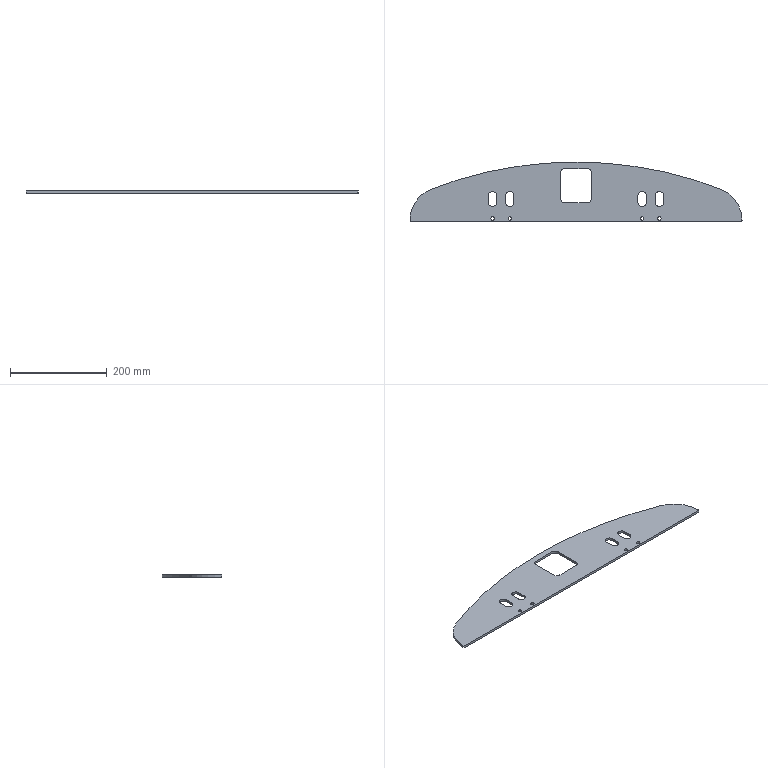Part | SolidWorks | features ICE 3, Fillet 1, FlatPattern 1, SMBaseFlange 1, SheetMetal 1 | 1 solid | 39 faces | box 688.178 x 124 x 5 mm | volume 305727 mm3 | cylinder 24 | plane 15 | commonest cylinder face diameters 7 x8 17 x8 20 x4 138.091 x3 1660 x1
STEP:
#1=CARTESIAN_POINT('',(230.5,7.,-5.));
#2=VERTEX_POINT('',#1);
#3=CARTESIAN_POINT('',(223.5,7.,-5.));
#4=VERTEX_POINT('',#3);
#5=CARTESIAN_POINT('',(227.,7.,-5.));
#6=DIRECTION('',(0.,0.,-1.));
#7=DIRECTION('',(-1.,0.,0.));
#8=AXIS2_PLACEMENT_3D('',#5,#6,#7);
#9=CIRCLE('',#8,3.5);
#10=EDGE_CURVE('',#2,#4,#9,.T.);
#11=ORIENTED_EDGE('',*,*,#10,.T.);
#12=CARTESIAN_POINT('',(223.5,7.,0.));
#13=VERTEX_POINT('',#12);
#14=CARTESIAN_POINT('',(223.5,7.,-10.));
#15=DIRECTION('',(0.,0.,1.));
#16=VECTOR('',#15,1000.);
#17=LINE('',#14,#16);
#18=EDGE_CURVE('',#4,#13,#17,.T.);
#19=ORIENTED_EDGE('',*,*,#18,.T.);
#20=CARTESIAN_POINT('',(230.5,7.,0.));
#21=VERTEX_POINT('',#20);
#22=CARTESIAN_POINT('',(227.,7.,0.));
#23=DIRECTION('',(0.,0.,1.));
#24=DIRECTION('',(1.,0.,0.));
#25=AXIS2_PLACEMENT_3D('',#22,#23,#24);
#26=CIRCLE('',#25,3.5);
#27=EDGE_CURVE('',#13,#21,#26,.T.);
#28=ORIENTED_EDGE('',*,*,#27,.T.);
#29=CARTESIAN_POINT('',(230.5,7.,-10.));
#30=DIRECTION('',(0.,0.,1.));
#31=VECTOR('',#30,1000.);
#32=LINE('',#29,#31);
#33=EDGE_CURVE('',#2,#21,#32,.T.);
#34=ORIENTED_EDGE('',*,*,#33,.F.);
#35=EDGE_LOOP('',(#11,#19,#28,#34));
#36=FACE_OUTER_BOUND('',#35,.T.);
#37=CARTESIAN_POINT('',(227.,7.,-10.));
#38=DIRECTION('',(0.,0.,1.));
#39=DIRECTION('',(1.,0.,0.));
#40=AXIS2_PLACEMENT_3D('',#37,#38,#39);
#41=CYLINDRICAL_SURFACE('',#40,3.5);
#42=ADVANCED_FACE('',(#36),#41,.F.);
#43=CARTESIAN_POINT('',(266.5,7.,-5.));
#44=VERTEX_POINT('',#43);
#45=CARTESIAN_POINT('',(259.5,7.,-5.));
#46=VERTEX_POINT('',#45);
#47=CARTESIAN_POINT('',(263.,7.,-5.));
#48=DIRECTION('',(0.,0.,-1.));
#49=DIRECTION('',(-1.,0.,0.));
#50=AXIS2_PLACEMENT_3D('',#47,#48,#49);
#51=CIRCLE('',#50,3.5);
#52=EDGE_CURVE('',#44,#46,#51,.T.);
#53=ORIENTED_EDGE('',*,*,#52,.T.);
#54=CARTESIAN_POINT('',(259.5,7.,0.));
#55=VERTEX_POINT('',#54);
#56=CARTESIAN_POINT('',(259.5,7.,-10.));
#57=DIRECTION('',(0.,0.,1.));
#58=VECTOR('',#57,1000.);
#59=LINE('',#56,#58);
#60=EDGE_CURVE('',#46,#55,#59,.T.);
#61=ORIENTED_EDGE('',*,*,#60,.T.);
#62=CARTESIAN_POINT('',(266.5,7.,0.));
#63=VERTEX_POINT('',#62);
#64=CARTESIAN_POINT('',(263.,7.,0.));
#65=DIRECTION('',(0.,0.,1.));
#66=DIRECTION('',(1.,0.,0.));
#67=AXIS2_PLACEMENT_3D('',#64,#65,#66);
#68=CIRCLE('',#67,3.5);
#69=EDGE_CURVE('',#55,#63,#68,.T.);
#70=ORIENTED_EDGE('',*,*,#69,.T.);
#71=CARTESIAN_POINT('',(266.5,7.,-10.));
#72=DIRECTION('',(0.,0.,1.));
#73=VECTOR('',#72,1000.);
#74=LINE('',#71,#73);
#75=EDGE_CURVE('',#44,#63,#74,.T.);
#76=ORIENTED_EDGE('',*,*,#75,.F.);
#77=EDGE_LOOP('',(#53,#61,#70,#76));
#78=FACE_OUTER_BOUND('',#77,.T.);
#79=CARTESIAN_POINT('',(263.,7.,-10.));
#80=DIRECTION('',(0.,0.,1.));
#81=DIRECTION('',(1.,0.,0.));
#82=AXIS2_PLACEMENT_3D('',#79,#80,#81);
#83=CYLINDRICAL_SURFACE('',#82,3.5);
#84=ADVANCED_FACE('',(#78),#83,.F.);
#85=CARTESIAN_POINT('',(540.5,7.,-5.));
#86=VERTEX_POINT('',#85);
#87=CARTESIAN_POINT('',(533.5,7.,-5.));
#88=VERTEX_POINT('',#87);
#89=CARTESIAN_POINT('',(537.,7.,-5.));
#90=DIRECTION('',(0.,0.,-1.));
#91=DIRECTION('',(-1.,0.,0.));
#92=AXIS2_PLACEMENT_3D('',#89,#90,#91);
#93=CIRCLE('',#92,3.5);
#94=EDGE_CURVE('',#86,#88,#93,.T.);
#95=ORIENTED_EDGE('',*,*,#94,.T.);
#96=CARTESIAN_POINT('',(533.5,7.,0.));
#97=VERTEX_POINT('',#96);
#98=CARTESIAN_POINT('',(533.5,7.,-10.));
#99=DIRECTION('',(0.,0.,1.));
#100=VECTOR('',#99,1000.);
#101=LINE('',#98,#100);
#102=EDGE_CURVE('',#88,#97,#101,.T.);
#103=ORIENTED_EDGE('',*,*,#102,.T.);
#104=CARTESIAN_POINT('',(540.5,7.,0.));
#105=VERTEX_POINT('',#104);
#106=CARTESIAN_POINT('',(537.,7.,0.));
#107=DIRECTION('',(0.,0.,1.));
#108=DIRECTION('',(-1.,0.,0.));
#109=AXIS2_PLACEMENT_3D('',#106,#107,#108);
#110=CIRCLE('',#109,3.5);
#111=EDGE_CURVE('',#97,#105,#110,.T.);
#112=ORIENTED_EDGE('',*,*,#111,.T.);
#113=CARTESIAN_POINT('',(540.5,7.,-10.));
#114=DIRECTION('',(0.,0.,1.));
#115=VECTOR('',#114,1000.);
#116=LINE('',#113,#115);
#117=EDGE_CURVE('',#86,#105,#116,.T.);
#118=ORIENTED_EDGE('',*,*,#117,.F.);
#119=EDGE_LOOP('',(#95,#103,#112,#118));
#120=FACE_OUTER_BOUND('',#119,.T.);
#121=CARTESIAN_POINT('',(537.,7.,-10.));
#122=DIRECTION('',(0.,0.,1.));
#123=DIRECTION('',(1.,0.,0.));
#124=AXIS2_PLACEMENT_3D('',#121,#122,#123);
#125=CYLINDRICAL_SURFACE('',#124,3.5);
#126=ADVANCED_FACE('',(#120),#125,.F.);
#127=CARTESIAN_POINT('',(576.5,7.,-5.));
#128=VERTEX_POINT('',#127);
#129=CARTESIAN_POINT('',(569.5,7.,-5.));
#130=VERTEX_POINT('',#129);
#131=CARTESIAN_POINT('',(573.,7.,-5.));
#132=DIRECTION('',(0.,0.,-1.));
#133=DIRECTION('',(-1.,0.,0.));
#134=AXIS2_PLACEMENT_3D('',#131,#132,#133);
#135=CIRCLE('',#134,3.5);
#136=EDGE_CURVE('',#128,#130,#135,.T.);
#137=ORIENTED_EDGE('',*,*,#136,.T.);
#138=CARTESIAN_POINT('',(569.5,7.,0.));
#139=VERTEX_POINT('',#138);
#140=CARTESIAN_POINT('',(569.5,7.,-10.));
#141=DIRECTION('',(0.,0.,1.));
#142=VECTOR('',#141,1000.);
#143=LINE('',#140,#142);
#144=EDGE_CURVE('',#130,#139,#143,.T.);
#145=ORIENTED_EDGE('',*,*,#144,.T.);
#146=CARTESIAN_POINT('',(576.5,7.,0.));
#147=VERTEX_POINT('',#146);
#148=CARTESIAN_POINT('',(573.,7.,0.));
#149=DIRECTION('',(0.,0.,1.));
#150=DIRECTION('',(-1.,0.,0.));
#151=AXIS2_PLACEMENT_3D('',#148,#149,#150);
#152=CIRCLE('',#151,3.5);
#153=EDGE_CURVE('',#139,#147,#152,.T.);
#154=ORIENTED_EDGE('',*,*,#153,.T.);
#155=CARTESIAN_POINT('',(576.5,7.,-10.));
#156=DIRECTION('',(0.,0.,1.));
#157=VECTOR('',#156,1000.);
#158=LINE('',#155,#157);
#159=EDGE_CURVE('',#128,#147,#158,.T.);
#160=ORIENTED_EDGE('',*,*,#159,.F.);
#161=EDGE_LOOP('',(#137,#145,#154,#160));
#162=FACE_OUTER_BOUND('',#161,.T.);
#163=CARTESIAN_POINT('',(573.,7.,-10.));
#164=DIRECTION('',(0.,0.,1.));
#165=DIRECTION('',(1.,0.,0.));
#166=AXIS2_PLACEMENT_3D('',#163,#164,#165);
#167=CYLINDRICAL_SURFACE('',#166,3.5);
#168=ADVANCED_FACE('',(#162),#167,.F.);
#169=CARTESIAN_POINT('',(744.,0.,-5.));
#170=VERTEX_POINT('',#169);
#171=CARTESIAN_POINT('',(744.089,3.509,-5.));
#172=VERTEX_POINT('',#171);
#173=CARTESIAN_POINT('',(675.044,3.509,-5.));
#174=DIRECTION('',(0.,0.,1.));
#175=DIRECTION('',(1.,0.,0.));
#176=AXIS2_PLACEMENT_3D('',#173,#174,#175);
#177=CIRCLE('',#176,69.045);
#178=EDGE_CURVE('',#170,#172,#177,.T.);
#179=ORIENTED_EDGE('',*,*,#178,.T.);
#180=CARTESIAN_POINT('',(744.089,3.509,0.));
#181=VERTEX_POINT('',#180);
#182=CARTESIAN_POINT('',(744.089,3.509,-5.));
#183=DIRECTION('',(0.,0.,1.));
#184=VECTOR('',#183,1000.);
#185=LINE('',#182,#184);
#186=EDGE_CURVE('',#172,#181,#185,.T.);
#187=ORIENTED_EDGE('',*,*,#186,.T.);
#188=CARTESIAN_POINT('',(744.,0.,0.));
#189=VERTEX_POINT('',#188);
#190=CARTESIAN_POINT('',(675.044,3.509,0.));
#191=DIRECTION('',(0.,0.,1.));
#192=DIRECTION('',(1.,0.,0.));
#193=AXIS2_PLACEMENT_3D('',#190,#191,#192);
#194=CIRCLE('',#193,69.045);
#195=EDGE_CURVE('',#189,#181,#194,.T.);
#196=ORIENTED_EDGE('',*,*,#195,.F.);
#197=CARTESIAN_POINT('',(744.,0.,-5.));
#198=DIRECTION('',(0.,0.,1.));
#199=VECTOR('',#198,1000.);
#200=LINE('',#197,#199);
#201=EDGE_CURVE('',#170,#189,#200,.T.);
#202=ORIENTED_EDGE('',*,*,#201,.F.);
#203=EDGE_LOOP('',(#179,#187,#196,#202));
#204=FACE_OUTER_BOUND('',#203,.T.);
#205=CARTESIAN_POINT('',(675.044,3.509,-5.));
#206=DIRECTION('',(0.,0.,1.));
#207=DIRECTION('',(1.,0.,0.));
#208=AXIS2_PLACEMENT_3D('',#205,#206,#207);
#209=CYLINDRICAL_SURFACE('',#208,69.045);
#210=ADVANCED_FACE('',(#204),#209,.T.);
#211=CARTESIAN_POINT('',(100.,67.886,0.));
#212=VERTEX_POINT('',#211);
#213=CARTESIAN_POINT('',(56.,0.,0.));
#214=VERTEX_POINT('',#213);
#215=CARTESIAN_POINT('',(124.956,3.509,0.));
#216=DIRECTION('',(0.,0.,1.));
#217=DIRECTION('',(-1.,0.,0.));
#218=AXIS2_PLACEMENT_3D('',#215,#216,#217);
#219=CIRCLE('',#218,69.045);
#220=EDGE_CURVE('',#212,#214,#219,.T.);
#221=ORIENTED_EDGE('',*,*,#220,.F.);
#222=CARTESIAN_POINT('',(100.,67.886,-5.));
#223=VERTEX_POINT('',#222);
#224=CARTESIAN_POINT('',(100.,67.886,-5.));
#225=DIRECTION('',(0.,0.,1.));
#226=VECTOR('',#225,1000.);
#227=LINE('',#224,#226);
#228=EDGE_CURVE('',#223,#212,#227,.T.);
#229=ORIENTED_EDGE('',*,*,#228,.F.);
#230=CARTESIAN_POINT('',(56.,0.,-5.));
#231=VERTEX_POINT('',#230);
#232=CARTESIAN_POINT('',(124.956,3.509,-5.));
#233=DIRECTION('',(0.,0.,1.));
#234=DIRECTION('',(-1.,0.,0.));
#235=AXIS2_PLACEMENT_3D('',#232,#233,#234);
#236=CIRCLE('',#235,69.045);
#237=EDGE_CURVE('',#223,#231,#236,.T.);
#238=ORIENTED_EDGE('',*,*,#237,.T.);
#239=CARTESIAN_POINT('',(56.,0.,-5.));
#240=DIRECTION('',(0.,0.,1.));
#241=VECTOR('',#240,1000.);
#242=LINE('',#239,#241);
#243=EDGE_CURVE('',#231,#214,#242,.T.);
#244=ORIENTED_EDGE('',*,*,#243,.T.);
#245=EDGE_LOOP('',(#221,#229,#238,#244));
#246=FACE_OUTER_BOUND('',#245,.T.);
#247=CARTESIAN_POINT('',(124.956,3.509,-5.));
#248=DIRECTION('',(0.,0.,1.));
#249=DIRECTION('',(1.,0.,0.));
#250=AXIS2_PLACEMENT_3D('',#247,#248,#249);
#251=CYLINDRICAL_SURFACE('',#250,69.045);
#252=ADVANCED_FACE('',(#246),#251,.T.);
#253=CARTESIAN_POINT('',(700.,67.886,0.));
#254=VERTEX_POINT('',#253);
#255=CARTESIAN_POINT('',(400.,-706.,0.));
#256=DIRECTION('',(0.,0.,1.));
#257=DIRECTION('',(-1.,0.,0.));
#258=AXIS2_PLACEMENT_3D('',#255,#256,#257);
#259=CIRCLE('',#258,830.);
#260=EDGE_CURVE('',#254,#212,#259,.T.);
#261=ORIENTED_EDGE('',*,*,#260,.F.);
#262=CARTESIAN_POINT('',(700.,67.886,-5.));
#263=VERTEX_POINT('',#262);
#264=CARTESIAN_POINT('',(700.,67.886,-5.));
#265=DIRECTION('',(0.,0.,1.));
#266=VECTOR('',#265,1000.);
#267=LINE('',#264,#266);
#268=EDGE_CURVE('',#263,#254,#267,.T.);
#269=ORIENTED_EDGE('',*,*,#268,.F.);
#270=CARTESIAN_POINT('',(400.,-706.,-5.));
#271=DIRECTION('',(0.,0.,1.));
#272=DIRECTION('',(-1.,0.,0.));
#273=AXIS2_PLACEMENT_3D('',#270,#271,#272);
#274=CIRCLE('',#273,830.);
#275=EDGE_CURVE('',#263,#223,#274,.T.);
#276=ORIENTED_EDGE('',*,*,#275,.T.);
#277=ORIENTED_EDGE('',*,*,#228,.T.);
#278=EDGE_LOOP('',(#261,#269,#276,#277));
#279=FACE_OUTER_BOUND('',#278,.T.);
#280=CARTESIAN_POINT('',(400.,-706.,-5.));
#281=DIRECTION('',(0.,0.,1.));
#282=DIRECTION('',(1.,0.,0.));
#283=AXIS2_PLACEMENT_3D('',#280,#281,#282);
#284=CYLINDRICAL_SURFACE('',#283,830.);
#285=ADVANCED_FACE('',(#279),#284,.T.);
#286=ORIENTED_EDGE('',*,*,#186,.F.);
#287=CARTESIAN_POINT('',(675.044,3.509,-5.));
#288=DIRECTION('',(0.,0.,1.));
#289=DIRECTION('',(1.,0.,0.));
#290=AXIS2_PLACEMENT_3D('',#287,#288,#289);
#291=CIRCLE('',#290,69.045);
#292=EDGE_CURVE('',#172,#263,#291,.T.);
#293=ORIENTED_EDGE('',*,*,#292,.T.);
#294=ORIENTED_EDGE('',*,*,#268,.T.);
#295=CARTESIAN_POINT('',(675.044,3.509,0.));
#296=DIRECTION('',(0.,0.,1.));
#297=DIRECTION('',(1.,0.,0.));
#298=AXIS2_PLACEMENT_3D('',#295,#296,#297);
#299=CIRCLE('',#298,69.045);
#300=EDGE_CURVE('',#181,#254,#299,.T.);
#301=ORIENTED_EDGE('',*,*,#300,.F.);
#302=EDGE_LOOP('',(#286,#293,#294,#301));
#303=FACE_OUTER_BOUND('',#302,.T.);
#304=CARTESIAN_POINT('',(675.044,3.509,-5.));
#305=DIRECTION('',(0.,0.,1.));
#306=DIRECTION('',(1.,0.,0.));
#307=AXIS2_PLACEMENT_3D('',#304,#305,#306);
#308=CYLINDRICAL_SURFACE('',#307,69.045);
#309=ADVANCED_FACE('',(#303),#308,.T.);
#310=CARTESIAN_POINT('',(56.,0.,0.));
#311=DIRECTION('',(1.,0.,0.));
#312=VECTOR('',#311,1000.);
#313=LINE('',#310,#312);
#314=EDGE_CURVE('',#214,#189,#313,.T.);
#315=ORIENTED_EDGE('',*,*,#314,.F.);
#316=ORIENTED_EDGE('',*,*,#243,.F.);
#317=CARTESIAN_POINT('',(56.,0.,-5.));
#318=DIRECTION('',(1.,0.,0.));
#319=VECTOR('',#318,1000.);
#320=LINE('',#317,#319);
#321=EDGE_CURVE('',#231,#170,#320,.T.);
#322=ORIENTED_EDGE('',*,*,#321,.T.);
#323=ORIENTED_EDGE('',*,*,#201,.T.);
#324=EDGE_LOOP('',(#315,#316,#322,#323));
#325=FACE_OUTER_BOUND('',#324,.T.);
#326=CARTESIAN_POINT('',(56.,0.,-5.));
#327=DIRECTION('',(0.,-1.,0.));
#328=DIRECTION('',(0.,0.,-1.));
#329=AXIS2_PLACEMENT_3D('',#326,#327,#328);
#330=PLANE('',#329);
#331=ADVANCED_FACE('',(#325),#330,.T.);
#332=ORIENTED_EDGE('',*,*,#10,.F.);
#333=CARTESIAN_POINT('',(227.,7.,-5.));
#334=DIRECTION('',(0.,0.,-1.));
#335=DIRECTION('',(-1.,0.,0.));
#336=AXIS2_PLACEMENT_3D('',#333,#334,#335);
#337=CIRCLE('',#336,3.5);
#338=EDGE_CURVE('',#4,#2,#337,.T.);
#339=ORIENTED_EDGE('',*,*,#338,.F.);
#340=EDGE_LOOP('',(#332,#339));
#341=FACE_BOUND('',#340,.T.);
#342=ORIENTED_EDGE('',*,*,#52,.F.);
#343=CARTESIAN_POINT('',(263.,7.,-5.));
#344=DIRECTION('',(0.,0.,-1.));
#345=DIRECTION('',(-1.,0.,0.));
#346=AXIS2_PLACEMENT_3D('',#343,#344,#345);
#347=CIRCLE('',#346,3.5);
#348=EDGE_CURVE('',#46,#44,#347,.T.);
#349=ORIENTED_EDGE('',*,*,#348,.F.);
#350=EDGE_LOOP('',(#342,#349));
#351=FACE_BOUND('',#350,.T.);
#352=ORIENTED_EDGE('',*,*,#94,.F.);
#353=CARTESIAN_POINT('',(537.,7.,-5.));
#354=DIRECTION('',(0.,0.,-1.));
#355=DIRECTION('',(-1.,0.,0.));
#356=AXIS2_PLACEMENT_3D('',#353,#354,#355);
#357=CIRCLE('',#356,3.5);
#358=EDGE_CURVE('',#88,#86,#357,.T.);
#359=ORIENTED_EDGE('',*,*,#358,.F.);
#360=EDGE_LOOP('',(#352,#359));
#361=FACE_BOUND('',#360,.T.);
#362=ORIENTED_EDGE('',*,*,#136,.F.);
#363=CARTESIAN_POINT('',(573.,7.,-5.));
#364=DIRECTION('',(0.,0.,-1.));
#365=DIRECTION('',(-1.,0.,0.));
#366=AXIS2_PLACEMENT_3D('',#363,#364,#365);
#367=CIRCLE('',#366,3.5);
#368=EDGE_CURVE('',#130,#128,#367,.T.);
#369=ORIENTED_EDGE('',*,*,#368,.F.);
#370=EDGE_LOOP('',(#362,#369));
#371=FACE_BOUND('',#370,.T.);
#372=CARTESIAN_POINT('',(218.5,40.,-5.));
#373=VERTEX_POINT('',#372);
#374=CARTESIAN_POINT('',(235.5,40.,-5.));
#375=VERTEX_POINT('',#374);
#376=CARTESIAN_POINT('',(227.,40.,-5.));
#377=DIRECTION('',(0.,0.,1.));
#378=DIRECTION('',(1.,0.,0.));
#379=AXIS2_PLACEMENT_3D('',#376,#377,#378);
#380=CIRCLE('',#379,8.5);
#381=EDGE_CURVE('',#373,#375,#380,.T.);
#382=ORIENTED_EDGE('',*,*,#381,.T.);
#383=CARTESIAN_POINT('',(235.5,55.,-5.));
#384=VERTEX_POINT('',#383);
#385=CARTESIAN_POINT('',(235.5,40.,-5.));
#386=DIRECTION('',(0.,1.,0.));
#387=VECTOR('',#386,1000.);
#388=LINE('',#385,#387);
#389=EDGE_CURVE('',#375,#384,#388,.T.);
#390=ORIENTED_EDGE('',*,*,#389,.T.);
#391=CARTESIAN_POINT('',(218.5,55.,-5.));
#392=VERTEX_POINT('',#391);
#393=CARTESIAN_POINT('',(227.,55.,-5.));
#394=DIRECTION('',(0.,0.,1.));
#395=DIRECTION('',(1.,0.,0.));
#396=AXIS2_PLACEMENT_3D('',#393,#394,#395);
#397=CIRCLE('',#396,8.5);
#398=EDGE_CURVE('',#384,#392,#397,.T.);
#399=ORIENTED_EDGE('',*,*,#398,.T.);
#400=CARTESIAN_POINT('',(218.5,40.,-5.));
#401=DIRECTION('',(0.,-1.,0.));
#402=VECTOR('',#401,1000.);
#403=LINE('',#400,#402);
#404=EDGE_CURVE('',#392,#373,#403,.T.);
#405=ORIENTED_EDGE('',*,*,#404,.T.);
#406=EDGE_LOOP('',(#382,#390,#399,#405));
#407=FACE_BOUND('',#406,.T.);
#408=CARTESIAN_POINT('',(528.5,40.,-5.));
#409=VERTEX_POINT('',#408);
#410=CARTESIAN_POINT('',(545.5,40.,-5.));
#411=VERTEX_POINT('',#410);
#412=CARTESIAN_POINT('',(537.,40.,-5.));
#413=DIRECTION('',(0.,0.,1.));
#414=DIRECTION('',(-1.,0.,0.));
#415=AXIS2_PLACEMENT_3D('',#412,#413,#414);
#416=CIRCLE('',#415,8.5);
#417=EDGE_CURVE('',#409,#411,#416,.T.);
#418=ORIENTED_EDGE('',*,*,#417,.T.);
#419=CARTESIAN_POINT('',(545.5,55.,-5.));
#420=VERTEX_POINT('',#419);
#421=CARTESIAN_POINT('',(545.5,40.,-5.));
#422=DIRECTION('',(0.,1.,0.));
#423=VECTOR('',#422,1000.);
#424=LINE('',#421,#423);
#425=EDGE_CURVE('',#411,#420,#424,.T.);
#426=ORIENTED_EDGE('',*,*,#425,.T.);
#427=CARTESIAN_POINT('',(528.5,55.,-5.));
#428=VERTEX_POINT('',#427);
#429=CARTESIAN_POINT('',(537.,55.,-5.));
#430=DIRECTION('',(0.,0.,1.));
#431=DIRECTION('',(-1.,0.,0.));
#432=AXIS2_PLACEMENT_3D('',#429,#430,#431);
#433=CIRCLE('',#432,8.5);
#434=EDGE_CURVE('',#420,#428,#433,.T.);
#435=ORIENTED_EDGE('',*,*,#434,.T.);
#436=CARTESIAN_POINT('',(528.5,40.,-5.));
#437=DIRECTION('',(0.,-1.,0.));
#438=VECTOR('',#437,1000.);
#439=LINE('',#436,#438);
#440=EDGE_CURVE('',#428,#409,#439,.T.);
#441=ORIENTED_EDGE('',*,*,#440,.T.);
#442=EDGE_LOOP('',(#418,#426,#435,#441));
#443=FACE_BOUND('',#442,.T.);
#444=CARTESIAN_POINT('',(564.5,40.,-5.));
#445=VERTEX_POINT('',#444);
#446=CARTESIAN_POINT('',(581.5,40.,-5.));
#447=VERTEX_POINT('',#446);
#448=CARTESIAN_POINT('',(573.,40.,-5.));
#449=DIRECTION('',(0.,0.,1.));
#450=DIRECTION('',(-1.,0.,0.));
#451=AXIS2_PLACEMENT_3D('',#448,#449,#450);
#452=CIRCLE('',#451,8.5);
#453=EDGE_CURVE('',#445,#447,#452,.T.);
#454=ORIENTED_EDGE('',*,*,#453,.T.);
#455=CARTESIAN_POINT('',(581.5,55.,-5.));
#456=VERTEX_POINT('',#455);
#457=CARTESIAN_POINT('',(581.5,40.,-5.));
#458=DIRECTION('',(0.,1.,0.));
#459=VECTOR('',#458,1000.);
#460=LINE('',#457,#459);
#461=EDGE_CURVE('',#447,#456,#460,.T.);
#462=ORIENTED_EDGE('',*,*,#461,.T.);
#463=CARTESIAN_POINT('',(564.5,55.,-5.));
#464=VERTEX_POINT('',#463);
#465=CARTESIAN_POINT('',(573.,55.,-5.));
#466=DIRECTION('',(0.,0.,1.));
#467=DIRECTION('',(-1.,0.,0.));
#468=AXIS2_PLACEMENT_3D('',#465,#466,#467);
#469=CIRCLE('',#468,8.5);
#470=EDGE_CURVE('',#456,#464,#469,.T.);
#471=ORIENTED_EDGE('',*,*,#470,.T.);
#472=CARTESIAN_POINT('',(564.5,40.,-5.));
#473=DIRECTION('',(0.,-1.,0.));
#474=VECTOR('',#473,1000.);
#475=LINE('',#472,#474);
#476=EDGE_CURVE('',#464,#445,#475,.T.);
#477=ORIENTED_EDGE('',*,*,#476,.T.);
#478=EDGE_LOOP('',(#454,#462,#471,#477));
#479=FACE_BOUND('',#478,.T.);
#480=CARTESIAN_POINT('',(254.5,40.,-5.));
#481=VERTEX_POINT('',#480);
#482=CARTESIAN_POINT('',(271.5,40.,-5.));
#483=VERTEX_POINT('',#482);
#484=CARTESIAN_POINT('',(263.,40.,-5.));
#485=DIRECTION('',(0.,0.,1.));
#486=DIRECTION('',(1.,0.,0.));
#487=AXIS2_PLACEMENT_3D('',#484,#485,#486);
#488=CIRCLE('',#487,8.5);
#489=EDGE_CURVE('',#481,#483,#488,.T.);
#490=ORIENTED_EDGE('',*,*,#489,.T.);
#491=CARTESIAN_POINT('',(271.5,55.,-5.));
#492=VERTEX_POINT('',#491);
#493=CARTESIAN_POINT('',(271.5,40.,-5.));
#494=DIRECTION('',(0.,1.,0.));
#495=VECTOR('',#494,1000.);
#496=LINE('',#493,#495);
#497=EDGE_CURVE('',#483,#492,#496,.T.);
#498=ORIENTED_EDGE('',*,*,#497,.T.);
#499=CARTESIAN_POINT('',(254.5,55.,-5.));
#500=VERTEX_POINT('',#499);
#501=CARTESIAN_POINT('',(263.,55.,-5.));
#502=DIRECTION('',(0.,0.,1.));
#503=DIRECTION('',(1.,0.,0.));
#504=AXIS2_PLACEMENT_3D('',#501,#502,#503);
#505=CIRCLE('',#504,8.5);
#506=EDGE_CURVE('',#492,#500,#505,.T.);
#507=ORIENTED_EDGE('',*,*,#506,.T.);
#508=CARTESIAN_POINT('',(254.5,40.,-5.));
#509=DIRECTION('',(0.,-1.,0.));
#510=VECTOR('',#509,1000.);
#511=LINE('',#508,#510);
#512=EDGE_CURVE('',#500,#481,#511,.T.);
#513=ORIENTED_EDGE('',*,*,#512,.T.);
#514=EDGE_LOOP('',(#490,#498,#507,#513));
#515=FACE_BOUND('',#514,.T.);
#516=CARTESIAN_POINT('',(433.,100.,-5.));
#517=VERTEX_POINT('',#516);
#518=CARTESIAN_POINT('',(433.,50.,-5.));
#519=VERTEX_POINT('',#518);
#520=CARTESIAN_POINT('',(433.,3.509,-5.));
#521=DIRECTION('',(0.,-1.,0.));
#522=VECTOR('',#521,1000.);
#523=LINE('',#520,#522);
#524=EDGE_CURVE('',#517,#519,#523,.T.);
#525=ORIENTED_EDGE('',*,*,#524,.F.);
#526=CARTESIAN_POINT('',(423.,110.,-5.));
#527=VERTEX_POINT('',#526);
#528=CARTESIAN_POINT('',(423.,100.,-5.));
#529=DIRECTION('',(0.,0.,1.));
#530=DIRECTION('',(-1.,0.,0.));
#531=AXIS2_PLACEMENT_3D('',#528,#529,#530);
#532=CIRCLE('',#531,10.);
#533=EDGE_CURVE('',#517,#527,#532,.T.);
#534=ORIENTED_EDGE('',*,*,#533,.T.);
#535=CARTESIAN_POINT('',(377.,110.,-5.));
#536=VERTEX_POINT('',#535);
#537=CARTESIAN_POINT('',(124.956,110.,-5.));
#538=DIRECTION('',(1.,0.,0.));
#539=VECTOR('',#538,1000.);
#540=LINE('',#537,#539);
#541=EDGE_CURVE('',#536,#527,#540,.T.);
#542=ORIENTED_EDGE('',*,*,#541,.F.);
#543=CARTESIAN_POINT('',(367.,100.,-5.));
#544=VERTEX_POINT('',#543);
#545=CARTESIAN_POINT('',(377.,100.,-5.));
#546=DIRECTION('',(0.,0.,1.));
#547=DIRECTION('',(-1.,0.,0.));
#548=AXIS2_PLACEMENT_3D('',#545,#546,#547);
#549=CIRCLE('',#548,10.);
#550=EDGE_CURVE('',#536,#544,#549,.T.);
#551=ORIENTED_EDGE('',*,*,#550,.T.);
#552=CARTESIAN_POINT('',(367.,50.,-5.));
#553=VERTEX_POINT('',#552);
#554=CARTESIAN_POINT('',(367.,3.509,-5.));
#555=DIRECTION('',(0.,1.,0.));
#556=VECTOR('',#555,1000.);
#557=LINE('',#554,#556);
#558=EDGE_CURVE('',#553,#544,#557,.T.);
#559=ORIENTED_EDGE('',*,*,#558,.F.);
#560=CARTESIAN_POINT('',(377.,40.,-5.));
#561=VERTEX_POINT('',#560);
#562=CARTESIAN_POINT('',(377.,50.,-5.));
#563=DIRECTION('',(0.,0.,1.));
#564=DIRECTION('',(-1.,0.,0.));
#565=AXIS2_PLACEMENT_3D('',#562,#563,#564);
#566=CIRCLE('',#565,10.);
#567=EDGE_CURVE('',#553,#561,#566,.T.);
#568=ORIENTED_EDGE('',*,*,#567,.T.);
#569=CARTESIAN_POINT('',(423.,40.,-5.));
#570=VERTEX_POINT('',#569);
#571=CARTESIAN_POINT('',(124.956,40.,-5.));
#572=DIRECTION('',(-1.,0.,0.));
#573=VECTOR('',#572,1000.);
#574=LINE('',#571,#573);
#575=EDGE_CURVE('',#570,#561,#574,.T.);
#576=ORIENTED_EDGE('',*,*,#575,.F.);
#577=CARTESIAN_POINT('',(423.,50.,-5.));
#578=DIRECTION('',(0.,0.,1.));
#579=DIRECTION('',(-1.,0.,0.));
#580=AXIS2_PLACEMENT_3D('',#577,#578,#579);
#581=CIRCLE('',#580,10.);
#582=EDGE_CURVE('',#570,#519,#581,.T.);
#583=ORIENTED_EDGE('',*,*,#582,.T.);
#584=EDGE_LOOP('',(#525,#534,#542,#551,#559,#568,#576,#583));
#585=FACE_BOUND('',#584,.T.);
#586=ORIENTED_EDGE('',*,*,#237,.F.);
#587=ORIENTED_EDGE('',*,*,#275,.F.);
#588=ORIENTED_EDGE('',*,*,#292,.F.);
#589=ORIENTED_EDGE('',*,*,#178,.F.);
#590=ORIENTED_EDGE('',*,*,#321,.F.);
#591=EDGE_LOOP('',(#586,#587,#588,#589,#590));
#592=FACE_OUTER_BOUND('',#591,.T.);
#593=CARTESIAN_POINT('',(124.956,3.509,-5.));
#594=DIRECTION('',(0.,0.,-1.));
#595=DIRECTION('',(-1.,0.,0.));
#596=AXIS2_PLACEMENT_3D('',#593,#594,#595);
#597=PLANE('',#596);
#598=ADVANCED_FACE('',(#341,#351,#361,#371,#407,#443,#479,#515,#585,#592),#597,.T.);
#599=CARTESIAN_POINT('',(227.,7.,0.));
#600=DIRECTION('',(0.,0.,1.));
#601=DIRECTION('',(1.,0.,0.));
#602=AXIS2_PLACEMENT_3D('',#599,#600,#601);
#603=CIRCLE('',#602,3.5);
#604=EDGE_CURVE('',#21,#13,#603,.T.);
#605=ORIENTED_EDGE('',*,*,#604,.F.);
#606=ORIENTED_EDGE('',*,*,#27,.F.);
#607=EDGE_LOOP('',(#605,#606));
#608=FACE_BOUND('',#607,.T.);
#609=CARTESIAN_POINT('',(263.,7.,0.));
#610=DIRECTION('',(0.,0.,1.));
#611=DIRECTION('',(1.,0.,0.));
#612=AXIS2_PLACEMENT_3D('',#609,#610,#611);
#613=CIRCLE('',#612,3.5);
#614=EDGE_CURVE('',#63,#55,#613,.T.);
#615=ORIENTED_EDGE('',*,*,#614,.F.);
#616=ORIENTED_EDGE('',*,*,#69,.F.);
#617=EDGE_LOOP('',(#615,#616));
#618=FACE_BOUND('',#617,.T.);
#619=CARTESIAN_POINT('',(537.,7.,0.));
#620=DIRECTION('',(0.,0.,1.));
#621=DIRECTION('',(-1.,0.,0.));
#622=AXIS2_PLACEMENT_3D('',#619,#620,#621);
#623=CIRCLE('',#622,3.5);
#624=EDGE_CURVE('',#105,#97,#623,.T.);
#625=ORIENTED_EDGE('',*,*,#624,.F.);
#626=ORIENTED_EDGE('',*,*,#111,.F.);
#627=EDGE_LOOP('',(#625,#626));
#628=FACE_BOUND('',#627,.T.);
#629=CARTESIAN_POINT('',(573.,7.,0.));
#630=DIRECTION('',(0.,0.,1.));
#631=DIRECTION('',(-1.,0.,0.));
#632=AXIS2_PLACEMENT_3D('',#629,#630,#631);
#633=CIRCLE('',#632,3.5);
#634=EDGE_CURVE('',#147,#139,#633,.T.);
#635=ORIENTED_EDGE('',*,*,#634,.F.);
#636=ORIENTED_EDGE('',*,*,#153,.F.);
#637=EDGE_LOOP('',(#635,#636));
#638=FACE_BOUND('',#637,.T.);
#639=CARTESIAN_POINT('',(235.5,40.,0.));
#640=VERTEX_POINT('',#639);
#641=CARTESIAN_POINT('',(235.5,55.,0.));
#642=VERTEX_POINT('',#641);
#643=CARTESIAN_POINT('',(235.5,40.,0.));
#644=DIRECTION('',(0.,1.,0.));
#645=VECTOR('',#644,1000.);
#646=LINE('',#643,#645);
#647=EDGE_CURVE('',#640,#642,#646,.T.);
#648=ORIENTED_EDGE('',*,*,#647,.F.);
#649=CARTESIAN_POINT('',(218.5,40.,0.));
#650=VERTEX_POINT('',#649);
#651=CARTESIAN_POINT('',(227.,40.,0.));
#652=DIRECTION('',(0.,0.,1.));
#653=DIRECTION('',(1.,0.,0.));
#654=AXIS2_PLACEMENT_3D('',#651,#652,#653);
#655=CIRCLE('',#654,8.5);
#656=EDGE_CURVE('',#650,#640,#655,.T.);
#657=ORIENTED_EDGE('',*,*,#656,.F.);
#658=CARTESIAN_POINT('',(218.5,55.,0.));
#659=VERTEX_POINT('',#658);
#660=CARTESIAN_POINT('',(218.5,40.,0.));
#661=DIRECTION('',(0.,-1.,0.));
#662=VECTOR('',#661,1000.);
#663=LINE('',#660,#662);
#664=EDGE_CURVE('',#659,#650,#663,.T.);
#665=ORIENTED_EDGE('',*,*,#664,.F.);
#666=CARTESIAN_POINT('',(227.,55.,0.));
#667=DIRECTION('',(0.,0.,1.));
#668=DIRECTION('',(1.,0.,0.));
#669=AXIS2_PLACEMENT_3D('',#666,#667,#668);
#670=CIRCLE('',#669,8.5);
#671=EDGE_CURVE('',#642,#659,#670,.T.);
#672=ORIENTED_EDGE('',*,*,#671,.F.);
#673=EDGE_LOOP('',(#648,#657,#665,#672));
#674=FACE_BOUND('',#673,.T.);
#675=CARTESIAN_POINT('',(545.5,40.,0.));
#676=VERTEX_POINT('',#675);
#677=CARTESIAN_POINT('',(545.5,55.,0.));
#678=VERTEX_POINT('',#677);
#679=CARTESIAN_POINT('',(545.5,40.,0.));
#680=DIRECTION('',(0.,1.,0.));
#681=VECTOR('',#680,1000.);
#682=LINE('',#679,#681);
#683=EDGE_CURVE('',#676,#678,#682,.T.);
#684=ORIENTED_EDGE('',*,*,#683,.F.);
#685=CARTESIAN_POINT('',(528.5,40.,0.));
#686=VERTEX_POINT('',#685);
#687=CARTESIAN_POINT('',(537.,40.,0.));
#688=DIRECTION('',(0.,0.,1.));
#689=DIRECTION('',(-1.,0.,0.));
#690=AXIS2_PLACEMENT_3D('',#687,#688,#689);
#691=CIRCLE('',#690,8.5);
#692=EDGE_CURVE('',#686,#676,#691,.T.);
#693=ORIENTED_EDGE('',*,*,#692,.F.);
#694=CARTESIAN_POINT('',(528.5,55.,0.));
#695=VERTEX_POINT('',#694);
#696=CARTESIAN_POINT('',(528.5,40.,0.));
#697=DIRECTION('',(0.,-1.,0.));
#698=VECTOR('',#697,1000.);
#699=LINE('',#696,#698);
#700=EDGE_CURVE('',#695,#686,#699,.T.);
#701=ORIENTED_EDGE('',*,*,#700,.F.);
#702=CARTESIAN_POINT('',(537.,55.,0.));
#703=DIRECTION('',(0.,0.,1.));
#704=DIRECTION('',(-1.,0.,0.));
#705=AXIS2_PLACEMENT_3D('',#702,#703,#704);
#706=CIRCLE('',#705,8.5);
#707=EDGE_CURVE('',#678,#695,#706,.T.);
#708=ORIENTED_EDGE('',*,*,#707,.F.);
#709=EDGE_LOOP('',(#684,#693,#701,#708));
#710=FACE_BOUND('',#709,.T.);
#711=CARTESIAN_POINT('',(581.5,40.,0.));
#712=VERTEX_POINT('',#711);
#713=CARTESIAN_POINT('',(581.5,55.,0.));
#714=VERTEX_POINT('',#713);
#715=CARTESIAN_POINT('',(581.5,40.,0.));
#716=DIRECTION('',(0.,1.,0.));
#717=VECTOR('',#716,1000.);
#718=LINE('',#715,#717);
#719=EDGE_CURVE('',#712,#714,#718,.T.);
#720=ORIENTED_EDGE('',*,*,#719,.F.);
#721=CARTESIAN_POINT('',(564.5,40.,0.));
#722=VERTEX_POINT('',#721);
#723=CARTESIAN_POINT('',(573.,40.,0.));
#724=DIRECTION('',(0.,0.,1.));
#725=DIRECTION('',(-1.,0.,0.));
#726=AXIS2_PLACEMENT_3D('',#723,#724,#725);
#727=CIRCLE('',#726,8.5);
#728=EDGE_CURVE('',#722,#712,#727,.T.);
#729=ORIENTED_EDGE('',*,*,#728,.F.);
#730=CARTESIAN_POINT('',(564.5,55.,0.));
#731=VERTEX_POINT('',#730);
#732=CARTESIAN_POINT('',(564.5,40.,0.));
#733=DIRECTION('',(0.,-1.,0.));
#734=VECTOR('',#733,1000.);
#735=LINE('',#732,#734);
#736=EDGE_CURVE('',#731,#722,#735,.T.);
#737=ORIENTED_EDGE('',*,*,#736,.F.);
#738=CARTESIAN_POINT('',(573.,55.,0.));
#739=DIRECTION('',(0.,0.,1.));
#740=DIRECTION('',(-1.,0.,0.));
#741=AXIS2_PLACEMENT_3D('',#738,#739,#740);
#742=CIRCLE('',#741,8.5);
#743=EDGE_CURVE('',#714,#731,#742,.T.);
#744=ORIENTED_EDGE('',*,*,#743,.F.);
#745=EDGE_LOOP('',(#720,#729,#737,#744));
#746=FACE_BOUND('',#745,.T.);
#747=CARTESIAN_POINT('',(271.5,40.,0.));
#748=VERTEX_POINT('',#747);
#749=CARTESIAN_POINT('',(271.5,55.,0.));
#750=VERTEX_POINT('',#749);
#751=CARTESIAN_POINT('',(271.5,40.,0.));
#752=DIRECTION('',(0.,1.,0.));
#753=VECTOR('',#752,1000.);
#754=LINE('',#751,#753);
#755=EDGE_CURVE('',#748,#750,#754,.T.);
#756=ORIENTED_EDGE('',*,*,#755,.F.);
#757=CARTESIAN_POINT('',(254.5,40.,0.));
#758=VERTEX_POINT('',#757);
#759=CARTESIAN_POINT('',(263.,40.,0.));
#760=DIRECTION('',(0.,0.,1.));
#761=DIRECTION('',(1.,0.,0.));
#762=AXIS2_PLACEMENT_3D('',#759,#760,#761);
#763=CIRCLE('',#762,8.5);
#764=EDGE_CURVE('',#758,#748,#763,.T.);
#765=ORIENTED_EDGE('',*,*,#764,.F.);
#766=CARTESIAN_POINT('',(254.5,55.,0.));
#767=VERTEX_POINT('',#766);
#768=CARTESIAN_POINT('',(254.5,40.,0.));
#769=DIRECTION('',(0.,-1.,0.));
#770=VECTOR('',#769,1000.);
#771=LINE('',#768,#770);
#772=EDGE_CURVE('',#767,#758,#771,.T.);
#773=ORIENTED_EDGE('',*,*,#772,.F.);
#774=CARTESIAN_POINT('',(263.,55.,0.));
#775=DIRECTION('',(0.,0.,1.));
#776=DIRECTION('',(1.,0.,0.));
#777=AXIS2_PLACEMENT_3D('',#774,#775,#776);
#778=CIRCLE('',#777,8.5);
#779=EDGE_CURVE('',#750,#767,#778,.T.);
#780=ORIENTED_EDGE('',*,*,#779,.F.);
#781=EDGE_LOOP('',(#756,#765,#773,#780));
#782=FACE_BOUND('',#781,.T.);
#783=CARTESIAN_POINT('',(423.,110.,0.));
#784=VERTEX_POINT('',#783);
#785=CARTESIAN_POINT('',(377.,110.,0.));
#786=VERTEX_POINT('',#785);
#787=CARTESIAN_POINT('',(367.,110.,0.));
#788=DIRECTION('',(-1.,0.,0.));
#789=VECTOR('',#788,1000.);
#790=LINE('',#787,#789);
#791=EDGE_CURVE('',#784,#786,#790,.T.);
#792=ORIENTED_EDGE('',*,*,#791,.F.);
#793=CARTESIAN_POINT('',(433.,100.,0.));
#794=VERTEX_POINT('',#793);
#795=CARTESIAN_POINT('',(423.,100.,0.));
#796=DIRECTION('',(0.,0.,-1.));
#797=DIRECTION('',(-1.,0.,0.));
#798=AXIS2_PLACEMENT_3D('',#795,#796,#797);
#799=CIRCLE('',#798,10.);
#800=EDGE_CURVE('',#784,#794,#799,.T.);
#801=ORIENTED_EDGE('',*,*,#800,.T.);
#802=CARTESIAN_POINT('',(433.,50.,0.));
#803=VERTEX_POINT('',#802);
#804=CARTESIAN_POINT('',(433.,110.,0.));
#805=DIRECTION('',(0.,1.,0.));
#806=VECTOR('',#805,1000.);
#807=LINE('',#804,#806);
#808=EDGE_CURVE('',#803,#794,#807,.T.);
#809=ORIENTED_EDGE('',*,*,#808,.F.);
#810=CARTESIAN_POINT('',(423.,40.,0.));
#811=VERTEX_POINT('',#810);
#812=CARTESIAN_POINT('',(423.,50.,0.));
#813=DIRECTION('',(0.,0.,-1.));
#814=DIRECTION('',(-1.,0.,0.));
#815=AXIS2_PLACEMENT_3D('',#812,#813,#814);
#816=CIRCLE('',#815,10.);
#817=EDGE_CURVE('',#803,#811,#816,.T.);
#818=ORIENTED_EDGE('',*,*,#817,.T.);
#819=CARTESIAN_POINT('',(377.,40.,0.));
#820=VERTEX_POINT('',#819);
#821=CARTESIAN_POINT('',(367.,40.,0.));
#822=DIRECTION('',(1.,0.,0.));
#823=VECTOR('',#822,1000.);
#824=LINE('',#821,#823);
#825=EDGE_CURVE('',#820,#811,#824,.T.);
#826=ORIENTED_EDGE('',*,*,#825,.F.);
#827=CARTESIAN_POINT('',(367.,50.,0.));
#828=VERTEX_POINT('',#827);
#829=CARTESIAN_POINT('',(377.,50.,0.));
#830=DIRECTION('',(0.,0.,-1.));
#831=DIRECTION('',(-1.,0.,0.));
#832=AXIS2_PLACEMENT_3D('',#829,#830,#831);
#833=CIRCLE('',#832,10.);
#834=EDGE_CURVE('',#820,#828,#833,.T.);
#835=ORIENTED_EDGE('',*,*,#834,.T.);
#836=CARTESIAN_POINT('',(367.,100.,0.));
#837=VERTEX_POINT('',#836);
#838=CARTESIAN_POINT('',(367.,110.,0.));
#839=DIRECTION('',(0.,-1.,0.));
#840=VECTOR('',#839,1000.);
#841=LINE('',#838,#840);
#842=EDGE_CURVE('',#837,#828,#841,.T.);
#843=ORIENTED_EDGE('',*,*,#842,.F.);
#844=CARTESIAN_POINT('',(377.,100.,0.));
#845=DIRECTION('',(0.,0.,-1.));
#846=DIRECTION('',(-1.,0.,0.));
#847=AXIS2_PLACEMENT_3D('',#844,#845,#846);
#848=CIRCLE('',#847,10.);
#849=EDGE_CURVE('',#837,#786,#848,.T.);
#850=ORIENTED_EDGE('',*,*,#849,.T.);
#851=EDGE_LOOP('',(#792,#801,#809,#818,#826,#835,#843,#850));
#852=FACE_BOUND('',#851,.T.);
#853=ORIENTED_EDGE('',*,*,#220,.T.);
#854=ORIENTED_EDGE('',*,*,#314,.T.);
#855=ORIENTED_EDGE('',*,*,#195,.T.);
#856=ORIENTED_EDGE('',*,*,#300,.T.);
#857=ORIENTED_EDGE('',*,*,#260,.T.);
#858=EDGE_LOOP('',(#853,#854,#855,#856,#857));
#859=FACE_OUTER_BOUND('',#858,.T.);
#860=CARTESIAN_POINT('',(124.956,3.509,0.));
#861=DIRECTION('',(0.,0.,-1.));
#862=DIRECTION('',(-1.,0.,0.));
#863=AXIS2_PLACEMENT_3D('',#860,#861,#862);
#864=PLANE('',#863);
#865=ADVANCED_FACE('',(#608,#618,#628,#638,#674,#710,#746,#782,#852,#859),#864,.F.);
#866=ORIENTED_EDGE('',*,*,#524,.T.);
#867=CARTESIAN_POINT('',(433.,50.,0.));
#868=DIRECTION('',(0.,0.,1.));
#869=VECTOR('',#868,1000.);
#870=LINE('',#867,#869);
#871=EDGE_CURVE('',#519,#803,#870,.T.);
#872=ORIENTED_EDGE('',*,*,#871,.T.);
#873=ORIENTED_EDGE('',*,*,#808,.T.);
#874=CARTESIAN_POINT('',(433.,100.,-5.));
#875=DIRECTION('',(0.,0.,-1.));
#876=VECTOR('',#875,1000.);
#877=LINE('',#874,#876);
#878=EDGE_CURVE('',#794,#517,#877,.T.);
#879=ORIENTED_EDGE('',*,*,#878,.T.);
#880=EDGE_LOOP('',(#866,#872,#873,#879));
#881=FACE_OUTER_BOUND('',#880,.T.);
#882=CARTESIAN_POINT('',(433.,110.,-10.));
#883=DIRECTION('',(1.,0.,0.));
#884=DIRECTION('',(0.,0.,-1.));
#885=AXIS2_PLACEMENT_3D('',#882,#883,#884);
#886=PLANE('',#885);
#887=ADVANCED_FACE('',(#881),#886,.F.);
#888=ORIENTED_EDGE('',*,*,#825,.T.);
#889=CARTESIAN_POINT('',(423.,40.,-5.));
#890=DIRECTION('',(0.,0.,-1.));
#891=VECTOR('',#890,1000.);
#892=LINE('',#889,#891);
#893=EDGE_CURVE('',#811,#570,#892,.T.);
#894=ORIENTED_EDGE('',*,*,#893,.T.);
#895=ORIENTED_EDGE('',*,*,#575,.T.);
#896=CARTESIAN_POINT('',(377.,40.,0.));
#897=DIRECTION('',(0.,0.,1.));
#898=VECTOR('',#897,1000.);
#899=LINE('',#896,#898);
#900=EDGE_CURVE('',#561,#820,#899,.T.);
#901=ORIENTED_EDGE('',*,*,#900,.T.);
#902=EDGE_LOOP('',(#888,#894,#895,#901));
#903=FACE_OUTER_BOUND('',#902,.T.);
#904=CARTESIAN_POINT('',(367.,40.,-10.));
#905=DIRECTION('',(0.,-1.,0.));
#906=DIRECTION('',(0.,0.,-1.));
#907=AXIS2_PLACEMENT_3D('',#904,#905,#906);
#908=PLANE('',#907);
#909=ADVANCED_FACE('',(#903),#908,.F.);
#910=ORIENTED_EDGE('',*,*,#842,.T.);
#911=CARTESIAN_POINT('',(367.,50.,-5.));
#912=DIRECTION('',(0.,0.,-1.));
#913=VECTOR('',#912,1000.);
#914=LINE('',#911,#913);
#915=EDGE_CURVE('',#828,#553,#914,.T.);
#916=ORIENTED_EDGE('',*,*,#915,.T.);
#917=ORIENTED_EDGE('',*,*,#558,.T.);
#918=CARTESIAN_POINT('',(367.,100.,0.));
#919=DIRECTION('',(0.,0.,1.));
#920=VECTOR('',#919,1000.);
#921=LINE('',#918,#920);
#922=EDGE_CURVE('',#544,#837,#921,.T.);
#923=ORIENTED_EDGE('',*,*,#922,.T.);
#924=EDGE_LOOP('',(#910,#916,#917,#923));
#925=FACE_OUTER_BOUND('',#924,.T.);
#926=CARTESIAN_POINT('',(367.,110.,-10.));
#927=DIRECTION('',(-1.,0.,0.));
#928=DIRECTION('',(0.,0.,1.));
#929=AXIS2_PLACEMENT_3D('',#926,#927,#928);
#930=PLANE('',#929);
#931=ADVANCED_FACE('',(#925),#930,.F.);
#932=ORIENTED_EDGE('',*,*,#541,.T.);
#933=CARTESIAN_POINT('',(423.,110.,0.));
#934=DIRECTION('',(0.,0.,1.));
#935=VECTOR('',#934,1000.);
#936=LINE('',#933,#935);
#937=EDGE_CURVE('',#527,#784,#936,.T.);
#938=ORIENTED_EDGE('',*,*,#937,.T.);
#939=ORIENTED_EDGE('',*,*,#791,.T.);
#940=CARTESIAN_POINT('',(377.,110.,-5.));
#941=DIRECTION('',(0.,0.,-1.));
#942=VECTOR('',#941,1000.);
#943=LINE('',#940,#942);
#944=EDGE_CURVE('',#786,#536,#943,.T.);
#945=ORIENTED_EDGE('',*,*,#944,.T.);
#946=EDGE_LOOP('',(#932,#938,#939,#945));
#947=FACE_OUTER_BOUND('',#946,.T.);
#948=CARTESIAN_POINT('',(367.,110.,-10.));
#949=DIRECTION('',(0.,1.,0.));
#950=DIRECTION('',(0.,0.,1.));
#951=AXIS2_PLACEMENT_3D('',#948,#949,#950);
#952=PLANE('',#951);
#953=ADVANCED_FACE('',(#947),#952,.F.);
#954=ORIENTED_EDGE('',*,*,#582,.F.);
#955=ORIENTED_EDGE('',*,*,#893,.F.);
#956=ORIENTED_EDGE('',*,*,#817,.F.);
#957=ORIENTED_EDGE('',*,*,#871,.F.);
#958=EDGE_LOOP('',(#954,#955,#956,#957));
#959=FACE_OUTER_BOUND('',#958,.T.);
#960=CARTESIAN_POINT('',(423.,50.,-10.));
#961=DIRECTION('',(0.,0.,-1.));
#962=DIRECTION('',(-1.,0.,0.));
#963=AXIS2_PLACEMENT_3D('',#960,#961,#962);
#964=CYLINDRICAL_SURFACE('',#963,10.);
#965=ADVANCED_FACE('',(#959),#964,.F.);
#966=ORIENTED_EDGE('',*,*,#567,.F.);
#967=ORIENTED_EDGE('',*,*,#915,.F.);
#968=ORIENTED_EDGE('',*,*,#834,.F.);
#969=ORIENTED_EDGE('',*,*,#900,.F.);
#970=EDGE_LOOP('',(#966,#967,#968,#969));
#971=FACE_OUTER_BOUND('',#970,.T.);
#972=CARTESIAN_POINT('',(377.,50.,-10.));
#973=DIRECTION('',(0.,0.,-1.));
#974=DIRECTION('',(-1.,0.,0.));
#975=AXIS2_PLACEMENT_3D('',#972,#973,#974);
#976=CYLINDRICAL_SURFACE('',#975,10.);
#977=ADVANCED_FACE('',(#971),#976,.F.);
#978=ORIENTED_EDGE('',*,*,#533,.F.);
#979=ORIENTED_EDGE('',*,*,#878,.F.);
#980=ORIENTED_EDGE('',*,*,#800,.F.);
#981=ORIENTED_EDGE('',*,*,#937,.F.);
#982=EDGE_LOOP('',(#978,#979,#980,#981));
#983=FACE_OUTER_BOUND('',#982,.T.);
#984=CARTESIAN_POINT('',(423.,100.,-10.));
#985=DIRECTION('',(0.,0.,-1.));
#986=DIRECTION('',(-1.,0.,0.));
#987=AXIS2_PLACEMENT_3D('',#984,#985,#986);
#988=CYLINDRICAL_SURFACE('',#987,10.);
#989=ADVANCED_FACE('',(#983),#988,.F.);
#990=ORIENTED_EDGE('',*,*,#550,.F.);
#991=ORIENTED_EDGE('',*,*,#944,.F.);
#992=ORIENTED_EDGE('',*,*,#849,.F.);
#993=ORIENTED_EDGE('',*,*,#922,.F.);
#994=EDGE_LOOP('',(#990,#991,#992,#993));
#995=FACE_OUTER_BOUND('',#994,.T.);
#996=CARTESIAN_POINT('',(377.,100.,-10.));
#997=DIRECTION('',(0.,0.,-1.));
#998=DIRECTION('',(-1.,0.,0.));
#999=AXIS2_PLACEMENT_3D('',#996,#997,#998);
#1000=CYLINDRICAL_SURFACE('',#999,10.);
#1001=ADVANCED_FACE('',(#995),#1000,.F.);
#1002=ORIENTED_EDGE('',*,*,#764,.T.);
#1003=CARTESIAN_POINT('',(271.5,40.,-5.));
#1004=DIRECTION('',(0.,0.,1.));
#1005=VECTOR('',#1004,1000.);
#1006=LINE('',#1003,#1005);
#1007=EDGE_CURVE('',#483,#748,#1006,.T.);
#1008=ORIENTED_EDGE('',*,*,#1007,.F.);
#1009=ORIENTED_EDGE('',*,*,#489,.F.);
#1010=CARTESIAN_POINT('',(254.5,40.,-5.));
#1011=DIRECTION('',(0.,0.,1.));
#1012=VECTOR('',#1011,1000.);
#1013=LINE('',#1010,#1012);
#1014=EDGE_CURVE('',#481,#758,#1013,.T.);
#1015=ORIENTED_EDGE('',*,*,#1014,.T.);
#1016=EDGE_LOOP('',(#1002,#1008,#1009,#1015));
#1017=FACE_OUTER_BOUND('',#1016,.T.);
#1018=CARTESIAN_POINT('',(263.,40.,-5.));
#1019=DIRECTION('',(0.,0.,1.));
#1020=DIRECTION('',(1.,0.,0.));
#1021=AXIS2_PLACEMENT_3D('',#1018,#1019,#1020);
#1022=CYLINDRICAL_SURFACE('',#1021,8.5);
#1023=ADVANCED_FACE('',(#1017),#1022,.F.);
#1024=ORIENTED_EDGE('',*,*,#772,.T.);
#1025=ORIENTED_EDGE('',*,*,#1014,.F.);
#1026=ORIENTED_EDGE('',*,*,#512,.F.);
#1027=CARTESIAN_POINT('',(254.5,55.,-5.));
#1028=DIRECTION('',(0.,0.,1.));
#1029=VECTOR('',#1028,1000.);
#1030=LINE('',#1027,#1029);
#1031=EDGE_CURVE('',#500,#767,#1030,.T.);
#1032=ORIENTED_EDGE('',*,*,#1031,.T.);
#1033=EDGE_LOOP('',(#1024,#1025,#1026,#1032));
#1034=FACE_OUTER_BOUND('',#1033,.T.);
#1035=CARTESIAN_POINT('',(254.5,40.,-5.));
#1036=DIRECTION('',(-1.,0.,0.));
#1037=DIRECTION('',(0.,0.,1.));
#1038=AXIS2_PLACEMENT_3D('',#1035,#1036,#1037);
#1039=PLANE('',#1038);
#1040=ADVANCED_FACE('',(#1034),#1039,.F.);
#1041=ORIENTED_EDGE('',*,*,#779,.T.);
#1042=ORIENTED_EDGE('',*,*,#1031,.F.);
#1043=ORIENTED_EDGE('',*,*,#506,.F.);
#1044=CARTESIAN_POINT('',(271.5,55.,-5.));
#1045=DIRECTION('',(0.,0.,1.));
#1046=VECTOR('',#1045,1000.);
#1047=LINE('',#1044,#1046);
#1048=EDGE_CURVE('',#492,#750,#1047,.T.);
#1049=ORIENTED_EDGE('',*,*,#1048,.T.);
#1050=EDGE_LOOP('',(#1041,#1042,#1043,#1049));
#1051=FACE_OUTER_BOUND('',#1050,.T.);
#1052=CARTESIAN_POINT('',(263.,55.,-5.));
#1053=DIRECTION('',(0.,0.,1.));
#1054=DIRECTION('',(1.,0.,0.));
#1055=AXIS2_PLACEMENT_3D('',#1052,#1053,#1054);
#1056=CYLINDRICAL_SURFACE('',#1055,8.5);
#1057=ADVANCED_FACE('',(#1051),#1056,.F.);
#1058=ORIENTED_EDGE('',*,*,#755,.T.);
#1059=ORIENTED_EDGE('',*,*,#1048,.F.);
#1060=ORIENTED_EDGE('',*,*,#497,.F.);
#1061=ORIENTED_EDGE('',*,*,#1007,.T.);
#1062=EDGE_LOOP('',(#1058,#1059,#1060,#1061));
#1063=FACE_OUTER_BOUND('',#1062,.T.);
#1064=CARTESIAN_POINT('',(271.5,40.,-5.));
#1065=DIRECTION('',(1.,0.,0.));
#1066=DIRECTION('',(0.,0.,-1.));
#1067=AXIS2_PLACEMENT_3D('',#1064,#1065,#1066);
#1068=PLANE('',#1067);
#1069=ADVANCED_FACE('',(#1063),#1068,.F.);
#1070=ORIENTED_EDGE('',*,*,#728,.T.);
#1071=CARTESIAN_POINT('',(581.5,40.,-5.));
#1072=DIRECTION('',(0.,0.,1.));
#1073=VECTOR('',#1072,1000.);
#1074=LINE('',#1071,#1073);
#1075=EDGE_CURVE('',#447,#712,#1074,.T.);
#1076=ORIENTED_EDGE('',*,*,#1075,.F.);
#1077=ORIENTED_EDGE('',*,*,#453,.F.);
#1078=CARTESIAN_POINT('',(564.5,40.,-5.));
#1079=DIRECTION('',(0.,0.,1.));
#1080=VECTOR('',#1079,1000.);
#1081=LINE('',#1078,#1080);
#1082=EDGE_CURVE('',#445,#722,#1081,.T.);
#1083=ORIENTED_EDGE('',*,*,#1082,.T.);
#1084=EDGE_LOOP('',(#1070,#1076,#1077,#1083));
#1085=FACE_OUTER_BOUND('',#1084,.T.);
#1086=CARTESIAN_POINT('',(573.,40.,-5.));
#1087=DIRECTION('',(0.,0.,1.));
#1088=DIRECTION('',(1.,0.,0.));
#1089=AXIS2_PLACEMENT_3D('',#1086,#1087,#1088);
#1090=CYLINDRICAL_SURFACE('',#1089,8.5);
#1091=ADVANCED_FACE('',(#1085),#1090,.F.);
#1092=ORIENTED_EDGE('',*,*,#736,.T.);
#1093=ORIENTED_EDGE('',*,*,#1082,.F.);
#1094=ORIENTED_EDGE('',*,*,#476,.F.);
#1095=CARTESIAN_POINT('',(564.5,55.,-5.));
#1096=DIRECTION('',(0.,0.,1.));
#1097=VECTOR('',#1096,1000.);
#1098=LINE('',#1095,#1097);
#1099=EDGE_CURVE('',#464,#731,#1098,.T.);
#1100=ORIENTED_EDGE('',*,*,#1099,.T.);
#1101=EDGE_LOOP('',(#1092,#1093,#1094,#1100));
#1102=FACE_OUTER_BOUND('',#1101,.T.);
#1103=CARTESIAN_POINT('',(564.5,40.,-5.));
#1104=DIRECTION('',(-1.,0.,0.));
#1105=DIRECTION('',(0.,0.,1.));
#1106=AXIS2_PLACEMENT_3D('',#1103,#1104,#1105);
#1107=PLANE('',#1106);
#1108=ADVANCED_FACE('',(#1102),#1107,.F.);
#1109=ORIENTED_EDGE('',*,*,#743,.T.);
#1110=ORIENTED_EDGE('',*,*,#1099,.F.);
#1111=ORIENTED_EDGE('',*,*,#470,.F.);
#1112=CARTESIAN_POINT('',(581.5,55.,-5.));
#1113=DIRECTION('',(0.,0.,1.));
#1114=VECTOR('',#1113,1000.);
#1115=LINE('',#1112,#1114);
#1116=EDGE_CURVE('',#456,#714,#1115,.T.);
#1117=ORIENTED_EDGE('',*,*,#1116,.T.);
#1118=EDGE_LOOP('',(#1109,#1110,#1111,#1117));
#1119=FACE_OUTER_BOUND('',#1118,.T.);
#1120=CARTESIAN_POINT('',(573.,55.,-5.));
#1121=DIRECTION('',(0.,0.,1.));
#1122=DIRECTION('',(1.,0.,0.));
#1123=AXIS2_PLACEMENT_3D('',#1120,#1121,#1122);
#1124=CYLINDRICAL_SURFACE('',#1123,8.5);
#1125=ADVANCED_FACE('',(#1119),#1124,.F.);
#1126=ORIENTED_EDGE('',*,*,#719,.T.);
#1127=ORIENTED_EDGE('',*,*,#1116,.F.);
#1128=ORIENTED_EDGE('',*,*,#461,.F.);
#1129=ORIENTED_EDGE('',*,*,#1075,.T.);
#1130=EDGE_LOOP('',(#1126,#1127,#1128,#1129));
#1131=FACE_OUTER_BOUND('',#1130,.T.);
#1132=CARTESIAN_POINT('',(581.5,40.,-5.));
#1133=DIRECTION('',(1.,0.,0.));
#1134=DIRECTION('',(0.,0.,-1.));
#1135=AXIS2_PLACEMENT_3D('',#1132,#1133,#1134);
#1136=PLANE('',#1135);
#1137=ADVANCED_FACE('',(#1131),#1136,.F.);
#1138=ORIENTED_EDGE('',*,*,#692,.T.);
#1139=CARTESIAN_POINT('',(545.5,40.,-5.));
#1140=DIRECTION('',(0.,0.,1.));
#1141=VECTOR('',#1140,1000.);
#1142=LINE('',#1139,#1141);
#1143=EDGE_CURVE('',#411,#676,#1142,.T.);
#1144=ORIENTED_EDGE('',*,*,#1143,.F.);
#1145=ORIENTED_EDGE('',*,*,#417,.F.);
#1146=CARTESIAN_POINT('',(528.5,40.,-5.));
#1147=DIRECTION('',(0.,0.,1.));
#1148=VECTOR('',#1147,1000.);
#1149=LINE('',#1146,#1148);
#1150=EDGE_CURVE('',#409,#686,#1149,.T.);
#1151=ORIENTED_EDGE('',*,*,#1150,.T.);
#1152=EDGE_LOOP('',(#1138,#1144,#1145,#1151));
#1153=FACE_OUTER_BOUND('',#1152,.T.);
#1154=CARTESIAN_POINT('',(537.,40.,-5.));
#1155=DIRECTION('',(0.,0.,1.));
#1156=DIRECTION('',(1.,0.,0.));
#1157=AXIS2_PLACEMENT_3D('',#1154,#1155,#1156);
#1158=CYLINDRICAL_SURFACE('',#1157,8.5);
#1159=ADVANCED_FACE('',(#1153),#1158,.F.);
#1160=ORIENTED_EDGE('',*,*,#700,.T.);
#1161=ORIENTED_EDGE('',*,*,#1150,.F.);
#1162=ORIENTED_EDGE('',*,*,#440,.F.);
#1163=CARTESIAN_POINT('',(528.5,55.,-5.));
#1164=DIRECTION('',(0.,0.,1.));
#1165=VECTOR('',#1164,1000.);
#1166=LINE('',#1163,#1165);
#1167=EDGE_CURVE('',#428,#695,#1166,.T.);
#1168=ORIENTED_EDGE('',*,*,#1167,.T.);
#1169=EDGE_LOOP('',(#1160,#1161,#1162,#1168));
#1170=FACE_OUTER_BOUND('',#1169,.T.);
#1171=CARTESIAN_POINT('',(528.5,40.,-5.));
#1172=DIRECTION('',(-1.,0.,0.));
#1173=DIRECTION('',(0.,0.,1.));
#1174=AXIS2_PLACEMENT_3D('',#1171,#1172,#1173);
#1175=PLANE('',#1174);
#1176=ADVANCED_FACE('',(#1170),#1175,.F.);
#1177=ORIENTED_EDGE('',*,*,#707,.T.);
#1178=ORIENTED_EDGE('',*,*,#1167,.F.);
#1179=ORIENTED_EDGE('',*,*,#434,.F.);
#1180=CARTESIAN_POINT('',(545.5,55.,-5.));
#1181=DIRECTION('',(0.,0.,1.));
#1182=VECTOR('',#1181,1000.);
#1183=LINE('',#1180,#1182);
#1184=EDGE_CURVE('',#420,#678,#1183,.T.);
#1185=ORIENTED_EDGE('',*,*,#1184,.T.);
#1186=EDGE_LOOP('',(#1177,#1178,#1179,#1185));
#1187=FACE_OUTER_BOUND('',#1186,.T.);
#1188=CARTESIAN_POINT('',(537.,55.,-5.));
#1189=DIRECTION('',(0.,0.,1.));
#1190=DIRECTION('',(1.,0.,0.));
#1191=AXIS2_PLACEMENT_3D('',#1188,#1189,#1190);
#1192=CYLINDRICAL_SURFACE('',#1191,8.5);
#1193=ADVANCED_FACE('',(#1187),#1192,.F.);
#1194=ORIENTED_EDGE('',*,*,#683,.T.);
#1195=ORIENTED_EDGE('',*,*,#1184,.F.);
#1196=ORIENTED_EDGE('',*,*,#425,.F.);
#1197=ORIENTED_EDGE('',*,*,#1143,.T.);
#1198=EDGE_LOOP('',(#1194,#1195,#1196,#1197));
#1199=FACE_OUTER_BOUND('',#1198,.T.);
#1200=CARTESIAN_POINT('',(545.5,40.,-5.));
#1201=DIRECTION('',(1.,0.,0.));
#1202=DIRECTION('',(0.,0.,-1.));
#1203=AXIS2_PLACEMENT_3D('',#1200,#1201,#1202);
#1204=PLANE('',#1203);
#1205=ADVANCED_FACE('',(#1199),#1204,.F.);
#1206=ORIENTED_EDGE('',*,*,#656,.T.);
#1207=CARTESIAN_POINT('',(235.5,40.,-5.));
#1208=DIRECTION('',(0.,0.,1.));
#1209=VECTOR('',#1208,1000.);
#1210=LINE('',#1207,#1209);
#1211=EDGE_CURVE('',#375,#640,#1210,.T.);
#1212=ORIENTED_EDGE('',*,*,#1211,.F.);
#1213=ORIENTED_EDGE('',*,*,#381,.F.);
#1214=CARTESIAN_POINT('',(218.5,40.,-5.));
#1215=DIRECTION('',(0.,0.,1.));
#1216=VECTOR('',#1215,1000.);
#1217=LINE('',#1214,#1216);
#1218=EDGE_CURVE('',#373,#650,#1217,.T.);
#1219=ORIENTED_EDGE('',*,*,#1218,.T.);
#1220=EDGE_LOOP('',(#1206,#1212,#1213,#1219));
#1221=FACE_OUTER_BOUND('',#1220,.T.);
#1222=CARTESIAN_POINT('',(227.,40.,-5.));
#1223=DIRECTION('',(0.,0.,1.));
#1224=DIRECTION('',(1.,0.,0.));
#1225=AXIS2_PLACEMENT_3D('',#1222,#1223,#1224);
#1226=CYLINDRICAL_SURFACE('',#1225,8.5);
#1227=ADVANCED_FACE('',(#1221),#1226,.F.);
#1228=ORIENTED_EDGE('',*,*,#664,.T.);
#1229=ORIENTED_EDGE('',*,*,#1218,.F.);
#1230=ORIENTED_EDGE('',*,*,#404,.F.);
#1231=CARTESIAN_POINT('',(218.5,55.,-5.));
#1232=DIRECTION('',(0.,0.,1.));
#1233=VECTOR('',#1232,1000.);
#1234=LINE('',#1231,#1233);
#1235=EDGE_CURVE('',#392,#659,#1234,.T.);
#1236=ORIENTED_EDGE('',*,*,#1235,.T.);
#1237=EDGE_LOOP('',(#1228,#1229,#1230,#1236));
#1238=FACE_OUTER_BOUND('',#1237,.T.);
#1239=CARTESIAN_POINT('',(218.5,40.,-5.));
#1240=DIRECTION('',(-1.,0.,0.));
#1241=DIRECTION('',(0.,-1.,0.));
#1242=AXIS2_PLACEMENT_3D('',#1239,#1240,#1241);
#1243=PLANE('',#1242);
#1244=ADVANCED_FACE('',(#1238),#1243,.F.);
#1245=ORIENTED_EDGE('',*,*,#671,.T.);
#1246=ORIENTED_EDGE('',*,*,#1235,.F.);
#1247=ORIENTED_EDGE('',*,*,#398,.F.);
#1248=CARTESIAN_POINT('',(235.5,55.,-5.));
#1249=DIRECTION('',(0.,0.,1.));
#1250=VECTOR('',#1249,1000.);
#1251=LINE('',#1248,#1250);
#1252=EDGE_CURVE('',#384,#642,#1251,.T.);
#1253=ORIENTED_EDGE('',*,*,#1252,.T.);
#1254=EDGE_LOOP('',(#1245,#1246,#1247,#1253));
#1255=FACE_OUTER_BOUND('',#1254,.T.);
#1256=CARTESIAN_POINT('',(227.,55.,-5.));
#1257=DIRECTION('',(0.,0.,1.));
#1258=DIRECTION('',(1.,0.,0.));
#1259=AXIS2_PLACEMENT_3D('',#1256,#1257,#1258);
#1260=CYLINDRICAL_SURFACE('',#1259,8.5);
#1261=ADVANCED_FACE('',(#1255),#1260,.F.);
#1262=ORIENTED_EDGE('',*,*,#647,.T.);
#1263=ORIENTED_EDGE('',*,*,#1252,.F.);
#1264=ORIENTED_EDGE('',*,*,#389,.F.);
#1265=ORIENTED_EDGE('',*,*,#1211,.T.);
#1266=EDGE_LOOP('',(#1262,#1263,#1264,#1265));
#1267=FACE_OUTER_BOUND('',#1266,.T.);
#1268=CARTESIAN_POINT('',(235.5,40.,-5.));
#1269=DIRECTION('',(1.,0.,0.));
#1270=DIRECTION('',(0.,0.,-1.));
#1271=AXIS2_PLACEMENT_3D('',#1268,#1269,#1270);
#1272=PLANE('',#1271);
#1273=ADVANCED_FACE('',(#1267),#1272,.F.);
#1274=ORIENTED_EDGE('',*,*,#144,.F.);
#1275=ORIENTED_EDGE('',*,*,#368,.T.);
#1276=ORIENTED_EDGE('',*,*,#159,.T.);
#1277=ORIENTED_EDGE('',*,*,#634,.T.);
#1278=EDGE_LOOP('',(#1274,#1275,#1276,#1277));
#1279=FACE_OUTER_BOUND('',#1278,.T.);
#1280=CARTESIAN_POINT('',(573.,7.,-10.));
#1281=DIRECTION('',(0.,0.,1.));
#1282=DIRECTION('',(1.,0.,0.));
#1283=AXIS2_PLACEMENT_3D('',#1280,#1281,#1282);
#1284=CYLINDRICAL_SURFACE('',#1283,3.5);
#1285=ADVANCED_FACE('',(#1279),#1284,.F.);
#1286=ORIENTED_EDGE('',*,*,#102,.F.);
#1287=ORIENTED_EDGE('',*,*,#358,.T.);
#1288=ORIENTED_EDGE('',*,*,#117,.T.);
#1289=ORIENTED_EDGE('',*,*,#624,.T.);
#1290=EDGE_LOOP('',(#1286,#1287,#1288,#1289));
#1291=FACE_OUTER_BOUND('',#1290,.T.);
#1292=CARTESIAN_POINT('',(537.,7.,-10.));
#1293=DIRECTION('',(0.,0.,1.));
#1294=DIRECTION('',(1.,0.,0.));
#1295=AXIS2_PLACEMENT_3D('',#1292,#1293,#1294);
#1296=CYLINDRICAL_SURFACE('',#1295,3.5);
#1297=ADVANCED_FACE('',(#1291),#1296,.F.);
#1298=ORIENTED_EDGE('',*,*,#60,.F.);
#1299=ORIENTED_EDGE('',*,*,#348,.T.);
#1300=ORIENTED_EDGE('',*,*,#75,.T.);
#1301=ORIENTED_EDGE('',*,*,#614,.T.);
#1302=EDGE_LOOP('',(#1298,#1299,#1300,#1301));
#1303=FACE_OUTER_BOUND('',#1302,.T.);
#1304=CARTESIAN_POINT('',(263.,7.,-10.));
#1305=DIRECTION('',(0.,0.,1.));
#1306=DIRECTION('',(1.,0.,0.));
#1307=AXIS2_PLACEMENT_3D('',#1304,#1305,#1306);
#1308=CYLINDRICAL_SURFACE('',#1307,3.5);
#1309=ADVANCED_FACE('',(#1303),#1308,.F.);
#1310=ORIENTED_EDGE('',*,*,#18,.F.);
#1311=ORIENTED_EDGE('',*,*,#338,.T.);
#1312=ORIENTED_EDGE('',*,*,#33,.T.);
#1313=ORIENTED_EDGE('',*,*,#604,.T.);
#1314=EDGE_LOOP('',(#1310,#1311,#1312,#1313));
#1315=FACE_OUTER_BOUND('',#1314,.T.);
#1316=CARTESIAN_POINT('',(227.,7.,-10.));
#1317=DIRECTION('',(0.,0.,1.));
#1318=DIRECTION('',(1.,0.,0.));
#1319=AXIS2_PLACEMENT_3D('',#1316,#1317,#1318);
#1320=CYLINDRICAL_SURFACE('',#1319,3.5);
#1321=ADVANCED_FACE('',(#1315),#1320,.F.);
#1322=CLOSED_SHELL('',(#42,#84,#126,#168,#210,#252,#285,#309,#331,#598,#865,#887,#909,#931,#953,#965,#977,#989,#1001,#1023,#1040,#1057,#1069,#1091,#1108,#1125,#1137,#1159,#1176,#1193,#1205,#1227,#1244,#1261,#1273,#1285,#1297,#1309,#1321));
#1323=MANIFOLD_SOLID_BREP('',#1322);
#1324=CARTESIAN_POINT('',(0.,0.,0.));
#1325=DIRECTION('',(0.,0.,1.));
#1326=DIRECTION('',(1.,0.,0.));
#1327=AXIS2_PLACEMENT_3D('',#1324,#1325,#1326);
#1328=(LENGTH_UNIT()NAMED_UNIT(*)SI_UNIT(.MILLI.,.METRE.));
#1329=UNCERTAINTY_MEASURE_WITH_UNIT(LENGTH_MEASURE(0.00001),#1328,'','');
#1330=(NAMED_UNIT(*)PLANE_ANGLE_UNIT()SI_UNIT($,.RADIAN.));
#1331=(NAMED_UNIT(*)SI_UNIT($,.STERADIAN.)SOLID_ANGLE_UNIT());
#1332=(GEOMETRIC_REPRESENTATION_CONTEXT(3)GLOBAL_UNCERTAINTY_ASSIGNED_CONTEXT((#1329))GLOBAL_UNIT_ASSIGNED_CONTEXT((#1328,#1330,#1331))REPRESENTATION_CONTEXT('',''));
#1333=ADVANCED_BREP_SHAPE_REPRESENTATION('',(#1323,#1327),#1332);